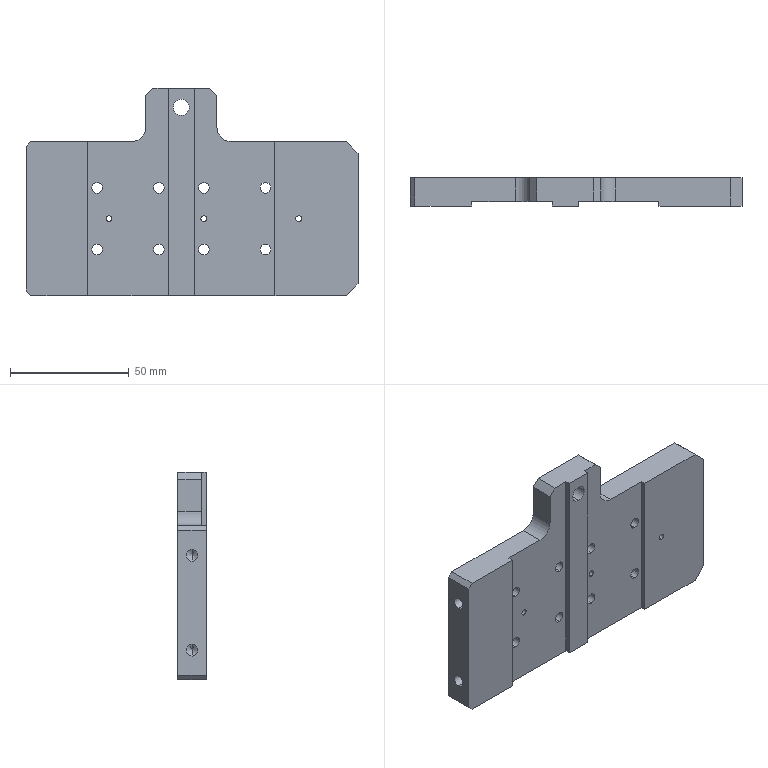Part | STEP file | PN_0040 | 1 solid | 88 faces | box 140 x 12 x 87.5 mm | volume 99789 mm3 | cylinder 48 | plane 36 | cone 4 | commonest cylinder face diameters 4.5 x16 8 x16 2.5 x6 5 x4 6.8 x2 10 x2